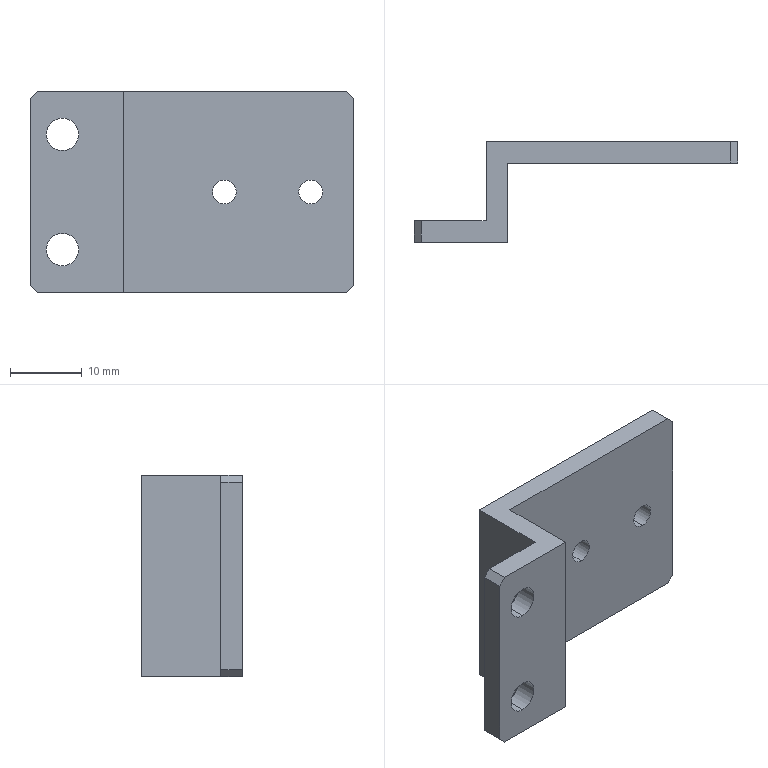Part | NX | features BREP 1 | 1 solid | 22 faces | box 45 x 14 x 28 mm | volume 4551 mm3 | plane 14 | cylinder 8 | commonest cylinder face diameters 3.3 x4 4.5 x4
STEP:
#1=CARTESIAN_POINT('',(103.864,-27.929,12.35));
#2=VERTEX_POINT('',#1);
#3=CARTESIAN_POINT('',(103.864,-27.929,15.65));
#4=VERTEX_POINT('',#3);
#5=CARTESIAN_POINT('',(103.864,-27.929,14.));
#6=DIRECTION('',(0.,1.,0.));
#7=DIRECTION('',(0.,0.,1.));
#8=AXIS2_PLACEMENT_3D('',#5,#6,#7);
#9=CIRCLE('',#8,1.65);
#10=EDGE_CURVE('',#2,#4,#9,.T.);
#11=ORIENTED_EDGE('',*,*,#10,.F.);
#12=CARTESIAN_POINT('',(103.864,-24.929,12.35));
#13=VERTEX_POINT('',#12);
#14=CARTESIAN_POINT('',(103.864,-24.929,12.35));
#15=DIRECTION('',(0.,1.,0.));
#16=VECTOR('',#15,1000.);
#17=LINE('',#14,#16);
#18=EDGE_CURVE('',#13,#2,#17,.F.);
#19=ORIENTED_EDGE('',*,*,#18,.F.);
#20=CARTESIAN_POINT('',(103.864,-24.929,15.65));
#21=VERTEX_POINT('',#20);
#22=CARTESIAN_POINT('',(103.864,-24.929,14.));
#23=DIRECTION('',(0.,1.,0.));
#24=DIRECTION('',(0.,0.,1.));
#25=AXIS2_PLACEMENT_3D('',#22,#23,#24);
#26=CIRCLE('',#25,1.65);
#27=EDGE_CURVE('',#13,#21,#26,.T.);
#28=ORIENTED_EDGE('',*,*,#27,.T.);
#29=CARTESIAN_POINT('',(103.864,-24.929,15.65));
#30=DIRECTION('',(0.,1.,0.));
#31=VECTOR('',#30,1000.);
#32=LINE('',#29,#31);
#33=EDGE_CURVE('',#21,#4,#32,.F.);
#34=ORIENTED_EDGE('',*,*,#33,.T.);
#35=EDGE_LOOP('',(#11,#19,#28,#34));
#36=FACE_BOUND('',#35,.T.);
#37=CARTESIAN_POINT('',(103.864,-24.929,14.));
#38=DIRECTION('',(0.,1.,0.));
#39=DIRECTION('',(0.,0.,1.));
#40=AXIS2_PLACEMENT_3D('',#37,#38,#39);
#41=CYLINDRICAL_SURFACE('',#40,1.65);
#42=ADVANCED_FACE('',(#36),#41,.F.);
#43=CARTESIAN_POINT('',(115.864,-27.929,12.35));
#44=VERTEX_POINT('',#43);
#45=CARTESIAN_POINT('',(115.864,-27.929,15.65));
#46=VERTEX_POINT('',#45);
#47=CARTESIAN_POINT('',(115.864,-27.929,14.));
#48=DIRECTION('',(0.,1.,0.));
#49=DIRECTION('',(0.,0.,1.));
#50=AXIS2_PLACEMENT_3D('',#47,#48,#49);
#51=CIRCLE('',#50,1.65);
#52=EDGE_CURVE('',#44,#46,#51,.T.);
#53=ORIENTED_EDGE('',*,*,#52,.F.);
#54=CARTESIAN_POINT('',(115.864,-24.929,12.35));
#55=VERTEX_POINT('',#54);
#56=CARTESIAN_POINT('',(115.864,-24.929,12.35));
#57=DIRECTION('',(0.,1.,0.));
#58=VECTOR('',#57,1000.);
#59=LINE('',#56,#58);
#60=EDGE_CURVE('',#55,#44,#59,.F.);
#61=ORIENTED_EDGE('',*,*,#60,.F.);
#62=CARTESIAN_POINT('',(115.864,-24.929,15.65));
#63=VERTEX_POINT('',#62);
#64=CARTESIAN_POINT('',(115.864,-24.929,14.));
#65=DIRECTION('',(0.,1.,0.));
#66=DIRECTION('',(0.,0.,1.));
#67=AXIS2_PLACEMENT_3D('',#64,#65,#66);
#68=CIRCLE('',#67,1.65);
#69=EDGE_CURVE('',#55,#63,#68,.T.);
#70=ORIENTED_EDGE('',*,*,#69,.T.);
#71=CARTESIAN_POINT('',(115.864,-24.929,15.65));
#72=DIRECTION('',(0.,1.,0.));
#73=VECTOR('',#72,1000.);
#74=LINE('',#71,#73);
#75=EDGE_CURVE('',#63,#46,#74,.F.);
#76=ORIENTED_EDGE('',*,*,#75,.T.);
#77=EDGE_LOOP('',(#53,#61,#70,#76));
#78=FACE_BOUND('',#77,.T.);
#79=CARTESIAN_POINT('',(115.864,-24.929,14.));
#80=DIRECTION('',(0.,1.,0.));
#81=DIRECTION('',(0.,0.,1.));
#82=AXIS2_PLACEMENT_3D('',#79,#80,#81);
#83=CYLINDRICAL_SURFACE('',#82,1.65);
#84=ADVANCED_FACE('',(#78),#83,.F.);
#85=CARTESIAN_POINT('',(81.364,-38.929,19.75));
#86=VERTEX_POINT('',#85);
#87=CARTESIAN_POINT('',(81.364,-38.929,24.25));
#88=VERTEX_POINT('',#87);
#89=CARTESIAN_POINT('',(81.364,-38.929,22.));
#90=DIRECTION('',(0.,1.,0.));
#91=DIRECTION('',(0.,0.,1.));
#92=AXIS2_PLACEMENT_3D('',#89,#90,#91);
#93=CIRCLE('',#92,2.25);
#94=EDGE_CURVE('',#86,#88,#93,.T.);
#95=ORIENTED_EDGE('',*,*,#94,.F.);
#96=CARTESIAN_POINT('',(81.364,-35.929,19.75));
#97=VERTEX_POINT('',#96);
#98=CARTESIAN_POINT('',(81.364,-38.929,19.75));
#99=DIRECTION('',(0.,1.,0.));
#100=VECTOR('',#99,1000.);
#101=LINE('',#98,#100);
#102=EDGE_CURVE('',#97,#86,#101,.F.);
#103=ORIENTED_EDGE('',*,*,#102,.F.);
#104=CARTESIAN_POINT('',(81.364,-35.929,24.25));
#105=VERTEX_POINT('',#104);
#106=CARTESIAN_POINT('',(81.364,-35.929,22.));
#107=DIRECTION('',(0.,1.,0.));
#108=DIRECTION('',(0.,0.,1.));
#109=AXIS2_PLACEMENT_3D('',#106,#107,#108);
#110=CIRCLE('',#109,2.25);
#111=EDGE_CURVE('',#97,#105,#110,.T.);
#112=ORIENTED_EDGE('',*,*,#111,.T.);
#113=CARTESIAN_POINT('',(81.364,-38.929,24.25));
#114=DIRECTION('',(0.,1.,0.));
#115=VECTOR('',#114,1000.);
#116=LINE('',#113,#115);
#117=EDGE_CURVE('',#105,#88,#116,.F.);
#118=ORIENTED_EDGE('',*,*,#117,.T.);
#119=EDGE_LOOP('',(#95,#103,#112,#118));
#120=FACE_BOUND('',#119,.T.);
#121=CARTESIAN_POINT('',(81.364,-38.929,22.));
#122=DIRECTION('',(0.,1.,0.));
#123=DIRECTION('',(0.,0.,1.));
#124=AXIS2_PLACEMENT_3D('',#121,#122,#123);
#125=CYLINDRICAL_SURFACE('',#124,2.25);
#126=ADVANCED_FACE('',(#120),#125,.F.);
#127=CARTESIAN_POINT('',(81.364,-38.929,3.75));
#128=VERTEX_POINT('',#127);
#129=CARTESIAN_POINT('',(81.364,-38.929,8.25));
#130=VERTEX_POINT('',#129);
#131=CARTESIAN_POINT('',(81.364,-38.929,6.));
#132=DIRECTION('',(0.,1.,0.));
#133=DIRECTION('',(0.,0.,1.));
#134=AXIS2_PLACEMENT_3D('',#131,#132,#133);
#135=CIRCLE('',#134,2.25);
#136=EDGE_CURVE('',#128,#130,#135,.T.);
#137=ORIENTED_EDGE('',*,*,#136,.F.);
#138=CARTESIAN_POINT('',(81.364,-35.929,3.75));
#139=VERTEX_POINT('',#138);
#140=CARTESIAN_POINT('',(81.364,-38.929,3.75));
#141=DIRECTION('',(0.,1.,0.));
#142=VECTOR('',#141,1000.);
#143=LINE('',#140,#142);
#144=EDGE_CURVE('',#139,#128,#143,.F.);
#145=ORIENTED_EDGE('',*,*,#144,.F.);
#146=CARTESIAN_POINT('',(81.364,-35.929,8.25));
#147=VERTEX_POINT('',#146);
#148=CARTESIAN_POINT('',(81.364,-35.929,6.));
#149=DIRECTION('',(0.,1.,0.));
#150=DIRECTION('',(0.,0.,1.));
#151=AXIS2_PLACEMENT_3D('',#148,#149,#150);
#152=CIRCLE('',#151,2.25);
#153=EDGE_CURVE('',#139,#147,#152,.T.);
#154=ORIENTED_EDGE('',*,*,#153,.T.);
#155=CARTESIAN_POINT('',(81.364,-38.929,8.25));
#156=DIRECTION('',(0.,1.,0.));
#157=VECTOR('',#156,1000.);
#158=LINE('',#155,#157);
#159=EDGE_CURVE('',#147,#130,#158,.F.);
#160=ORIENTED_EDGE('',*,*,#159,.T.);
#161=EDGE_LOOP('',(#137,#145,#154,#160));
#162=FACE_BOUND('',#161,.T.);
#163=CARTESIAN_POINT('',(81.364,-38.929,6.));
#164=DIRECTION('',(0.,1.,0.));
#165=DIRECTION('',(0.,0.,1.));
#166=AXIS2_PLACEMENT_3D('',#163,#164,#165);
#167=CYLINDRICAL_SURFACE('',#166,2.25);
#168=ADVANCED_FACE('',(#162),#167,.F.);
#169=CARTESIAN_POINT('',(86.864,-24.929,0.));
#170=VERTEX_POINT('',#169);
#171=CARTESIAN_POINT('',(86.864,-35.929,0.));
#172=VERTEX_POINT('',#171);
#173=CARTESIAN_POINT('',(86.864,-24.929,0.));
#174=DIRECTION('',(0.,-1.,0.));
#175=VECTOR('',#174,1000.);
#176=LINE('',#173,#175);
#177=EDGE_CURVE('',#170,#172,#176,.T.);
#178=ORIENTED_EDGE('',*,*,#177,.T.);
#179=CARTESIAN_POINT('',(86.864,-35.929,28.));
#180=VERTEX_POINT('',#179);
#181=CARTESIAN_POINT('',(86.864,-35.929,28.));
#182=DIRECTION('',(0.,0.,-1.));
#183=VECTOR('',#182,1000.);
#184=LINE('',#181,#183);
#185=EDGE_CURVE('',#180,#172,#184,.T.);
#186=ORIENTED_EDGE('',*,*,#185,.F.);
#187=CARTESIAN_POINT('',(86.864,-24.929,28.));
#188=VERTEX_POINT('',#187);
#189=CARTESIAN_POINT('',(86.864,-24.929,28.));
#190=DIRECTION('',(0.,-1.,0.));
#191=VECTOR('',#190,1000.);
#192=LINE('',#189,#191);
#193=EDGE_CURVE('',#188,#180,#192,.T.);
#194=ORIENTED_EDGE('',*,*,#193,.F.);
#195=CARTESIAN_POINT('',(86.864,-24.929,28.));
#196=DIRECTION('',(0.,0.,-1.));
#197=VECTOR('',#196,1000.);
#198=LINE('',#195,#197);
#199=EDGE_CURVE('',#188,#170,#198,.T.);
#200=ORIENTED_EDGE('',*,*,#199,.T.);
#201=EDGE_LOOP('',(#178,#186,#194,#200));
#202=FACE_BOUND('',#201,.T.);
#203=CARTESIAN_POINT('',(86.864,-24.929,28.));
#204=DIRECTION('',(1.,0.,0.));
#205=DIRECTION('',(0.,1.,0.));
#206=AXIS2_PLACEMENT_3D('',#203,#204,#205);
#207=PLANE('',#206);
#208=ADVANCED_FACE('',(#202),#207,.F.);
#209=CARTESIAN_POINT('',(77.864,-35.929,0.));
#210=VERTEX_POINT('',#209);
#211=CARTESIAN_POINT('',(86.864,-35.929,0.));
#212=DIRECTION('',(-1.,0.,0.));
#213=VECTOR('',#212,1000.);
#214=LINE('',#211,#213);
#215=EDGE_CURVE('',#172,#210,#214,.T.);
#216=ORIENTED_EDGE('',*,*,#215,.T.);
#217=CARTESIAN_POINT('',(76.864,-35.929,1.));
#218=VERTEX_POINT('',#217);
#219=CARTESIAN_POINT('',(76.864,-35.929,1.));
#220=DIRECTION('',(-0.7071,0.,0.7071));
#221=VECTOR('',#220,1000.);
#222=LINE('',#219,#221);
#223=EDGE_CURVE('',#210,#218,#222,.T.);
#224=ORIENTED_EDGE('',*,*,#223,.T.);
#225=CARTESIAN_POINT('',(76.864,-35.929,27.));
#226=VERTEX_POINT('',#225);
#227=CARTESIAN_POINT('',(76.864,-35.929,28.));
#228=DIRECTION('',(0.,0.,-1.));
#229=VECTOR('',#228,1000.);
#230=LINE('',#227,#229);
#231=EDGE_CURVE('',#226,#218,#230,.T.);
#232=ORIENTED_EDGE('',*,*,#231,.F.);
#233=CARTESIAN_POINT('',(77.864,-35.929,28.));
#234=VERTEX_POINT('',#233);
#235=CARTESIAN_POINT('',(77.864,-35.929,28.));
#236=DIRECTION('',(0.7071,0.,0.7071));
#237=VECTOR('',#236,1000.);
#238=LINE('',#235,#237);
#239=EDGE_CURVE('',#226,#234,#238,.T.);
#240=ORIENTED_EDGE('',*,*,#239,.T.);
#241=CARTESIAN_POINT('',(86.864,-35.929,28.));
#242=DIRECTION('',(-1.,0.,0.));
#243=VECTOR('',#242,1000.);
#244=LINE('',#241,#243);
#245=EDGE_CURVE('',#180,#234,#244,.T.);
#246=ORIENTED_EDGE('',*,*,#245,.F.);
#247=ORIENTED_EDGE('',*,*,#185,.T.);
#248=EDGE_LOOP('',(#216,#224,#232,#240,#246,#247));
#249=FACE_BOUND('',#248,.T.);
#250=CARTESIAN_POINT('',(81.364,-35.929,22.));
#251=DIRECTION('',(0.,1.,0.));
#252=DIRECTION('',(0.,0.,1.));
#253=AXIS2_PLACEMENT_3D('',#250,#251,#252);
#254=CIRCLE('',#253,2.25);
#255=EDGE_CURVE('',#105,#97,#254,.T.);
#256=ORIENTED_EDGE('',*,*,#255,.F.);
#257=ORIENTED_EDGE('',*,*,#111,.F.);
#258=EDGE_LOOP('',(#256,#257));
#259=FACE_BOUND('',#258,.T.);
#260=CARTESIAN_POINT('',(81.364,-35.929,6.));
#261=DIRECTION('',(0.,1.,0.));
#262=DIRECTION('',(0.,0.,1.));
#263=AXIS2_PLACEMENT_3D('',#260,#261,#262);
#264=CIRCLE('',#263,2.25);
#265=EDGE_CURVE('',#147,#139,#264,.T.);
#266=ORIENTED_EDGE('',*,*,#265,.F.);
#267=ORIENTED_EDGE('',*,*,#153,.F.);
#268=EDGE_LOOP('',(#266,#267));
#269=FACE_BOUND('',#268,.T.);
#270=CARTESIAN_POINT('',(86.864,-35.929,28.));
#271=DIRECTION('',(0.,-1.,0.));
#272=DIRECTION('',(0.,0.,-1.));
#273=AXIS2_PLACEMENT_3D('',#270,#271,#272);
#274=PLANE('',#273);
#275=ADVANCED_FACE('',(#249,#259,#269),#274,.F.);
#276=ORIENTED_EDGE('',*,*,#231,.T.);
#277=CARTESIAN_POINT('',(76.864,-38.929,1.));
#278=VERTEX_POINT('',#277);
#279=CARTESIAN_POINT('',(76.864,-38.929,1.));
#280=DIRECTION('',(0.,-1.,0.));
#281=VECTOR('',#280,1000.);
#282=LINE('',#279,#281);
#283=EDGE_CURVE('',#218,#278,#282,.T.);
#284=ORIENTED_EDGE('',*,*,#283,.T.);
#285=CARTESIAN_POINT('',(76.864,-38.929,27.));
#286=VERTEX_POINT('',#285);
#287=CARTESIAN_POINT('',(76.864,-38.929,28.));
#288=DIRECTION('',(0.,0.,-1.));
#289=VECTOR('',#288,1000.);
#290=LINE('',#287,#289);
#291=EDGE_CURVE('',#286,#278,#290,.T.);
#292=ORIENTED_EDGE('',*,*,#291,.F.);
#293=CARTESIAN_POINT('',(76.864,-35.929,27.));
#294=DIRECTION('',(0.,1.,0.));
#295=VECTOR('',#294,1000.);
#296=LINE('',#293,#295);
#297=EDGE_CURVE('',#286,#226,#296,.T.);
#298=ORIENTED_EDGE('',*,*,#297,.T.);
#299=EDGE_LOOP('',(#276,#284,#292,#298));
#300=FACE_BOUND('',#299,.T.);
#301=CARTESIAN_POINT('',(76.864,-35.929,28.));
#302=DIRECTION('',(1.,0.,0.));
#303=DIRECTION('',(0.,1.,0.));
#304=AXIS2_PLACEMENT_3D('',#301,#302,#303);
#305=PLANE('',#304);
#306=ADVANCED_FACE('',(#300),#305,.F.);
#307=ORIENTED_EDGE('',*,*,#291,.T.);
#308=CARTESIAN_POINT('',(77.864,-38.929,0.));
#309=VERTEX_POINT('',#308);
#310=CARTESIAN_POINT('',(76.864,-38.929,1.));
#311=DIRECTION('',(0.7071,0.,-0.7071));
#312=VECTOR('',#311,1000.);
#313=LINE('',#310,#312);
#314=EDGE_CURVE('',#278,#309,#313,.T.);
#315=ORIENTED_EDGE('',*,*,#314,.T.);
#316=CARTESIAN_POINT('',(89.864,-38.929,0.));
#317=VERTEX_POINT('',#316);
#318=CARTESIAN_POINT('',(89.864,-38.929,0.));
#319=DIRECTION('',(1.,0.,0.));
#320=VECTOR('',#319,1000.);
#321=LINE('',#318,#320);
#322=EDGE_CURVE('',#309,#317,#321,.T.);
#323=ORIENTED_EDGE('',*,*,#322,.T.);
#324=CARTESIAN_POINT('',(89.864,-38.929,28.));
#325=VERTEX_POINT('',#324);
#326=CARTESIAN_POINT('',(89.864,-38.929,28.));
#327=DIRECTION('',(0.,0.,-1.));
#328=VECTOR('',#327,1000.);
#329=LINE('',#326,#328);
#330=EDGE_CURVE('',#325,#317,#329,.T.);
#331=ORIENTED_EDGE('',*,*,#330,.F.);
#332=CARTESIAN_POINT('',(77.864,-38.929,28.));
#333=VERTEX_POINT('',#332);
#334=CARTESIAN_POINT('',(89.864,-38.929,28.));
#335=DIRECTION('',(1.,0.,0.));
#336=VECTOR('',#335,1000.);
#337=LINE('',#334,#336);
#338=EDGE_CURVE('',#333,#325,#337,.T.);
#339=ORIENTED_EDGE('',*,*,#338,.F.);
#340=CARTESIAN_POINT('',(77.864,-38.929,28.));
#341=DIRECTION('',(-0.7071,0.,-0.7071));
#342=VECTOR('',#341,1000.);
#343=LINE('',#340,#342);
#344=EDGE_CURVE('',#333,#286,#343,.T.);
#345=ORIENTED_EDGE('',*,*,#344,.T.);
#346=EDGE_LOOP('',(#307,#315,#323,#331,#339,#345));
#347=FACE_BOUND('',#346,.T.);
#348=CARTESIAN_POINT('',(81.364,-38.929,22.));
#349=DIRECTION('',(0.,1.,0.));
#350=DIRECTION('',(0.,0.,1.));
#351=AXIS2_PLACEMENT_3D('',#348,#349,#350);
#352=CIRCLE('',#351,2.25);
#353=EDGE_CURVE('',#88,#86,#352,.T.);
#354=ORIENTED_EDGE('',*,*,#353,.T.);
#355=ORIENTED_EDGE('',*,*,#94,.T.);
#356=EDGE_LOOP('',(#354,#355));
#357=FACE_BOUND('',#356,.T.);
#358=CARTESIAN_POINT('',(81.364,-38.929,6.));
#359=DIRECTION('',(0.,1.,0.));
#360=DIRECTION('',(0.,0.,1.));
#361=AXIS2_PLACEMENT_3D('',#358,#359,#360);
#362=CIRCLE('',#361,2.25);
#363=EDGE_CURVE('',#130,#128,#362,.T.);
#364=ORIENTED_EDGE('',*,*,#363,.T.);
#365=ORIENTED_EDGE('',*,*,#136,.T.);
#366=EDGE_LOOP('',(#364,#365));
#367=FACE_BOUND('',#366,.T.);
#368=CARTESIAN_POINT('',(89.864,-38.929,28.));
#369=DIRECTION('',(0.,1.,0.));
#370=DIRECTION('',(1.,0.,0.));
#371=AXIS2_PLACEMENT_3D('',#368,#369,#370);
#372=PLANE('',#371);
#373=ADVANCED_FACE('',(#347,#357,#367),#372,.F.);
#374=CARTESIAN_POINT('',(89.864,-27.929,0.));
#375=VERTEX_POINT('',#374);
#376=CARTESIAN_POINT('',(89.864,-27.929,0.));
#377=DIRECTION('',(0.,1.,0.));
#378=VECTOR('',#377,1000.);
#379=LINE('',#376,#378);
#380=EDGE_CURVE('',#317,#375,#379,.T.);
#381=ORIENTED_EDGE('',*,*,#380,.T.);
#382=CARTESIAN_POINT('',(89.864,-27.929,28.));
#383=VERTEX_POINT('',#382);
#384=CARTESIAN_POINT('',(89.864,-27.929,28.));
#385=DIRECTION('',(0.,0.,-1.));
#386=VECTOR('',#385,1000.);
#387=LINE('',#384,#386);
#388=EDGE_CURVE('',#383,#375,#387,.T.);
#389=ORIENTED_EDGE('',*,*,#388,.F.);
#390=CARTESIAN_POINT('',(89.864,-27.929,28.));
#391=DIRECTION('',(0.,1.,0.));
#392=VECTOR('',#391,1000.);
#393=LINE('',#390,#392);
#394=EDGE_CURVE('',#325,#383,#393,.T.);
#395=ORIENTED_EDGE('',*,*,#394,.F.);
#396=ORIENTED_EDGE('',*,*,#330,.T.);
#397=EDGE_LOOP('',(#381,#389,#395,#396));
#398=FACE_BOUND('',#397,.T.);
#399=CARTESIAN_POINT('',(89.864,-27.929,28.));
#400=DIRECTION('',(-1.,0.,0.));
#401=DIRECTION('',(0.,0.,1.));
#402=AXIS2_PLACEMENT_3D('',#399,#400,#401);
#403=PLANE('',#402);
#404=ADVANCED_FACE('',(#398),#403,.F.);
#405=CARTESIAN_POINT('',(120.864,-27.929,0.));
#406=VERTEX_POINT('',#405);
#407=CARTESIAN_POINT('',(89.864,-27.929,0.));
#408=DIRECTION('',(1.,0.,0.));
#409=VECTOR('',#408,1000.);
#410=LINE('',#407,#409);
#411=EDGE_CURVE('',#375,#406,#410,.T.);
#412=ORIENTED_EDGE('',*,*,#411,.T.);
#413=CARTESIAN_POINT('',(121.864,-27.929,1.));
#414=VERTEX_POINT('',#413);
#415=CARTESIAN_POINT('',(121.864,-27.929,1.));
#416=DIRECTION('',(0.7071,0.,0.7071));
#417=VECTOR('',#416,1000.);
#418=LINE('',#415,#417);
#419=EDGE_CURVE('',#406,#414,#418,.T.);
#420=ORIENTED_EDGE('',*,*,#419,.T.);
#421=CARTESIAN_POINT('',(121.864,-27.929,27.));
#422=VERTEX_POINT('',#421);
#423=CARTESIAN_POINT('',(121.864,-27.929,28.));
#424=DIRECTION('',(0.,0.,-1.));
#425=VECTOR('',#424,1000.);
#426=LINE('',#423,#425);
#427=EDGE_CURVE('',#422,#414,#426,.T.);
#428=ORIENTED_EDGE('',*,*,#427,.F.);
#429=CARTESIAN_POINT('',(120.864,-27.929,28.));
#430=VERTEX_POINT('',#429);
#431=CARTESIAN_POINT('',(120.864,-27.929,28.));
#432=DIRECTION('',(-0.7071,0.,0.7071));
#433=VECTOR('',#432,1000.);
#434=LINE('',#431,#433);
#435=EDGE_CURVE('',#422,#430,#434,.T.);
#436=ORIENTED_EDGE('',*,*,#435,.T.);
#437=CARTESIAN_POINT('',(89.864,-27.929,28.));
#438=DIRECTION('',(1.,0.,0.));
#439=VECTOR('',#438,1000.);
#440=LINE('',#437,#439);
#441=EDGE_CURVE('',#383,#430,#440,.T.);
#442=ORIENTED_EDGE('',*,*,#441,.F.);
#443=ORIENTED_EDGE('',*,*,#388,.T.);
#444=EDGE_LOOP('',(#412,#420,#428,#436,#442,#443));
#445=FACE_BOUND('',#444,.T.);
#446=CARTESIAN_POINT('',(103.864,-27.929,14.));
#447=DIRECTION('',(0.,1.,0.));
#448=DIRECTION('',(0.,0.,1.));
#449=AXIS2_PLACEMENT_3D('',#446,#447,#448);
#450=CIRCLE('',#449,1.65);
#451=EDGE_CURVE('',#4,#2,#450,.T.);
#452=ORIENTED_EDGE('',*,*,#451,.T.);
#453=ORIENTED_EDGE('',*,*,#10,.T.);
#454=EDGE_LOOP('',(#452,#453));
#455=FACE_BOUND('',#454,.T.);
#456=CARTESIAN_POINT('',(115.864,-27.929,14.));
#457=DIRECTION('',(0.,1.,0.));
#458=DIRECTION('',(0.,0.,1.));
#459=AXIS2_PLACEMENT_3D('',#456,#457,#458);
#460=CIRCLE('',#459,1.65);
#461=EDGE_CURVE('',#46,#44,#460,.T.);
#462=ORIENTED_EDGE('',*,*,#461,.T.);
#463=ORIENTED_EDGE('',*,*,#52,.T.);
#464=EDGE_LOOP('',(#462,#463));
#465=FACE_BOUND('',#464,.T.);
#466=CARTESIAN_POINT('',(89.864,-27.929,28.));
#467=DIRECTION('',(0.,1.,0.));
#468=DIRECTION('',(1.,0.,0.));
#469=AXIS2_PLACEMENT_3D('',#466,#467,#468);
#470=PLANE('',#469);
#471=ADVANCED_FACE('',(#445,#455,#465),#470,.F.);
#472=ORIENTED_EDGE('',*,*,#427,.T.);
#473=CARTESIAN_POINT('',(121.864,-24.929,1.));
#474=VERTEX_POINT('',#473);
#475=CARTESIAN_POINT('',(121.864,-24.929,1.));
#476=DIRECTION('',(0.,1.,0.));
#477=VECTOR('',#476,1000.);
#478=LINE('',#475,#477);
#479=EDGE_CURVE('',#414,#474,#478,.T.);
#480=ORIENTED_EDGE('',*,*,#479,.T.);
#481=CARTESIAN_POINT('',(121.864,-24.929,27.));
#482=VERTEX_POINT('',#481);
#483=CARTESIAN_POINT('',(121.864,-24.929,28.));
#484=DIRECTION('',(0.,0.,-1.));
#485=VECTOR('',#484,1000.);
#486=LINE('',#483,#485);
#487=EDGE_CURVE('',#482,#474,#486,.T.);
#488=ORIENTED_EDGE('',*,*,#487,.F.);
#489=CARTESIAN_POINT('',(121.864,-24.929,27.));
#490=DIRECTION('',(0.,-1.,0.));
#491=VECTOR('',#490,1000.);
#492=LINE('',#489,#491);
#493=EDGE_CURVE('',#482,#422,#492,.T.);
#494=ORIENTED_EDGE('',*,*,#493,.T.);
#495=EDGE_LOOP('',(#472,#480,#488,#494));
#496=FACE_BOUND('',#495,.T.);
#497=CARTESIAN_POINT('',(121.864,-24.929,28.));
#498=DIRECTION('',(-1.,0.,0.));
#499=DIRECTION('',(0.,0.,1.));
#500=AXIS2_PLACEMENT_3D('',#497,#498,#499);
#501=PLANE('',#500);
#502=ADVANCED_FACE('',(#496),#501,.F.);
#503=ORIENTED_EDGE('',*,*,#487,.T.);
#504=CARTESIAN_POINT('',(120.864,-24.929,0.));
#505=VERTEX_POINT('',#504);
#506=CARTESIAN_POINT('',(121.864,-24.929,1.));
#507=DIRECTION('',(-0.7071,0.,-0.7071));
#508=VECTOR('',#507,1000.);
#509=LINE('',#506,#508);
#510=EDGE_CURVE('',#474,#505,#509,.T.);
#511=ORIENTED_EDGE('',*,*,#510,.T.);
#512=CARTESIAN_POINT('',(86.864,-24.929,0.));
#513=DIRECTION('',(-1.,0.,0.));
#514=VECTOR('',#513,1000.);
#515=LINE('',#512,#514);
#516=EDGE_CURVE('',#505,#170,#515,.T.);
#517=ORIENTED_EDGE('',*,*,#516,.T.);
#518=ORIENTED_EDGE('',*,*,#199,.F.);
#519=CARTESIAN_POINT('',(120.864,-24.929,28.));
#520=VERTEX_POINT('',#519);
#521=CARTESIAN_POINT('',(86.864,-24.929,28.));
#522=DIRECTION('',(-1.,0.,0.));
#523=VECTOR('',#522,1000.);
#524=LINE('',#521,#523);
#525=EDGE_CURVE('',#520,#188,#524,.T.);
#526=ORIENTED_EDGE('',*,*,#525,.F.);
#527=CARTESIAN_POINT('',(120.864,-24.929,28.));
#528=DIRECTION('',(0.7071,0.,-0.7071));
#529=VECTOR('',#528,1000.);
#530=LINE('',#527,#529);
#531=EDGE_CURVE('',#520,#482,#530,.T.);
#532=ORIENTED_EDGE('',*,*,#531,.T.);
#533=EDGE_LOOP('',(#503,#511,#517,#518,#526,#532));
#534=FACE_BOUND('',#533,.T.);
#535=CARTESIAN_POINT('',(103.864,-24.929,14.));
#536=DIRECTION('',(0.,1.,0.));
#537=DIRECTION('',(0.,0.,1.));
#538=AXIS2_PLACEMENT_3D('',#535,#536,#537);
#539=CIRCLE('',#538,1.65);
#540=EDGE_CURVE('',#21,#13,#539,.T.);
#541=ORIENTED_EDGE('',*,*,#540,.F.);
#542=ORIENTED_EDGE('',*,*,#27,.F.);
#543=EDGE_LOOP('',(#541,#542));
#544=FACE_BOUND('',#543,.T.);
#545=CARTESIAN_POINT('',(115.864,-24.929,14.));
#546=DIRECTION('',(0.,1.,0.));
#547=DIRECTION('',(0.,0.,1.));
#548=AXIS2_PLACEMENT_3D('',#545,#546,#547);
#549=CIRCLE('',#548,1.65);
#550=EDGE_CURVE('',#63,#55,#549,.T.);
#551=ORIENTED_EDGE('',*,*,#550,.F.);
#552=ORIENTED_EDGE('',*,*,#69,.F.);
#553=EDGE_LOOP('',(#551,#552));
#554=FACE_BOUND('',#553,.T.);
#555=CARTESIAN_POINT('',(86.864,-24.929,28.));
#556=DIRECTION('',(0.,-1.,0.));
#557=DIRECTION('',(0.,0.,-1.));
#558=AXIS2_PLACEMENT_3D('',#555,#556,#557);
#559=PLANE('',#558);
#560=ADVANCED_FACE('',(#534,#544,#554),#559,.F.);
#561=ORIENTED_EDGE('',*,*,#441,.T.);
#562=CARTESIAN_POINT('',(120.864,-35.929,28.));
#563=DIRECTION('',(0.,1.,0.));
#564=VECTOR('',#563,1000.);
#565=LINE('',#562,#564);
#566=EDGE_CURVE('',#430,#520,#565,.T.);
#567=ORIENTED_EDGE('',*,*,#566,.T.);
#568=ORIENTED_EDGE('',*,*,#525,.T.);
#569=ORIENTED_EDGE('',*,*,#193,.T.);
#570=ORIENTED_EDGE('',*,*,#245,.T.);
#571=CARTESIAN_POINT('',(77.864,-35.929,28.));
#572=DIRECTION('',(0.,-1.,0.));
#573=VECTOR('',#572,1000.);
#574=LINE('',#571,#573);
#575=EDGE_CURVE('',#234,#333,#574,.T.);
#576=ORIENTED_EDGE('',*,*,#575,.T.);
#577=ORIENTED_EDGE('',*,*,#338,.T.);
#578=ORIENTED_EDGE('',*,*,#394,.T.);
#579=EDGE_LOOP('',(#561,#567,#568,#569,#570,#576,#577,#578));
#580=FACE_BOUND('',#579,.T.);
#581=CARTESIAN_POINT('',(86.864,-35.929,28.));
#582=DIRECTION('',(0.,0.,-1.));
#583=DIRECTION('',(0.,-1.,0.));
#584=AXIS2_PLACEMENT_3D('',#581,#582,#583);
#585=PLANE('',#584);
#586=ADVANCED_FACE('',(#580),#585,.F.);
#587=ORIENTED_EDGE('',*,*,#516,.F.);
#588=CARTESIAN_POINT('',(120.864,-27.929,0.));
#589=DIRECTION('',(0.,-1.,0.));
#590=VECTOR('',#589,1000.);
#591=LINE('',#588,#590);
#592=EDGE_CURVE('',#505,#406,#591,.T.);
#593=ORIENTED_EDGE('',*,*,#592,.T.);
#594=ORIENTED_EDGE('',*,*,#411,.F.);
#595=ORIENTED_EDGE('',*,*,#380,.F.);
#596=ORIENTED_EDGE('',*,*,#322,.F.);
#597=CARTESIAN_POINT('',(77.864,-35.929,0.));
#598=DIRECTION('',(0.,1.,0.));
#599=VECTOR('',#598,1000.);
#600=LINE('',#597,#599);
#601=EDGE_CURVE('',#309,#210,#600,.T.);
#602=ORIENTED_EDGE('',*,*,#601,.T.);
#603=ORIENTED_EDGE('',*,*,#215,.F.);
#604=ORIENTED_EDGE('',*,*,#177,.F.);
#605=EDGE_LOOP('',(#587,#593,#594,#595,#596,#602,#603,#604));
#606=FACE_BOUND('',#605,.T.);
#607=CARTESIAN_POINT('',(86.864,-35.929,0.));
#608=DIRECTION('',(0.,0.,-1.));
#609=DIRECTION('',(0.,-1.,0.));
#610=AXIS2_PLACEMENT_3D('',#607,#608,#609);
#611=PLANE('',#610);
#612=ADVANCED_FACE('',(#606),#611,.T.);
#613=ORIENTED_EDGE('',*,*,#144,.T.);
#614=ORIENTED_EDGE('',*,*,#363,.F.);
#615=ORIENTED_EDGE('',*,*,#159,.F.);
#616=ORIENTED_EDGE('',*,*,#265,.T.);
#617=EDGE_LOOP('',(#613,#614,#615,#616));
#618=FACE_BOUND('',#617,.T.);
#619=CARTESIAN_POINT('',(81.364,-38.929,6.));
#620=DIRECTION('',(0.,1.,0.));
#621=DIRECTION('',(0.,0.,1.));
#622=AXIS2_PLACEMENT_3D('',#619,#620,#621);
#623=CYLINDRICAL_SURFACE('',#622,2.25);
#624=ADVANCED_FACE('',(#618),#623,.F.);
#625=ORIENTED_EDGE('',*,*,#102,.T.);
#626=ORIENTED_EDGE('',*,*,#353,.F.);
#627=ORIENTED_EDGE('',*,*,#117,.F.);
#628=ORIENTED_EDGE('',*,*,#255,.T.);
#629=EDGE_LOOP('',(#625,#626,#627,#628));
#630=FACE_BOUND('',#629,.T.);
#631=CARTESIAN_POINT('',(81.364,-38.929,22.));
#632=DIRECTION('',(0.,1.,0.));
#633=DIRECTION('',(0.,0.,1.));
#634=AXIS2_PLACEMENT_3D('',#631,#632,#633);
#635=CYLINDRICAL_SURFACE('',#634,2.25);
#636=ADVANCED_FACE('',(#630),#635,.F.);
#637=ORIENTED_EDGE('',*,*,#60,.T.);
#638=ORIENTED_EDGE('',*,*,#461,.F.);
#639=ORIENTED_EDGE('',*,*,#75,.F.);
#640=ORIENTED_EDGE('',*,*,#550,.T.);
#641=EDGE_LOOP('',(#637,#638,#639,#640));
#642=FACE_BOUND('',#641,.T.);
#643=CARTESIAN_POINT('',(115.864,-24.929,14.));
#644=DIRECTION('',(0.,1.,0.));
#645=DIRECTION('',(0.,0.,1.));
#646=AXIS2_PLACEMENT_3D('',#643,#644,#645);
#647=CYLINDRICAL_SURFACE('',#646,1.65);
#648=ADVANCED_FACE('',(#642),#647,.F.);
#649=ORIENTED_EDGE('',*,*,#18,.T.);
#650=ORIENTED_EDGE('',*,*,#451,.F.);
#651=ORIENTED_EDGE('',*,*,#33,.F.);
#652=ORIENTED_EDGE('',*,*,#540,.T.);
#653=EDGE_LOOP('',(#649,#650,#651,#652));
#654=FACE_BOUND('',#653,.T.);
#655=CARTESIAN_POINT('',(103.864,-24.929,14.));
#656=DIRECTION('',(0.,1.,0.));
#657=DIRECTION('',(0.,0.,1.));
#658=AXIS2_PLACEMENT_3D('',#655,#656,#657);
#659=CYLINDRICAL_SURFACE('',#658,1.65);
#660=ADVANCED_FACE('',(#654),#659,.F.);
#661=ORIENTED_EDGE('',*,*,#419,.F.);
#662=ORIENTED_EDGE('',*,*,#592,.F.);
#663=ORIENTED_EDGE('',*,*,#510,.F.);
#664=ORIENTED_EDGE('',*,*,#479,.F.);
#665=EDGE_LOOP('',(#661,#662,#663,#664));
#666=FACE_BOUND('',#665,.T.);
#667=CARTESIAN_POINT('',(121.864,-24.929,1.));
#668=DIRECTION('',(0.7071,0.,-0.7071));
#669=DIRECTION('',(0.,-1.,0.));
#670=AXIS2_PLACEMENT_3D('',#667,#668,#669);
#671=PLANE('',#670);
#672=ADVANCED_FACE('',(#666),#671,.T.);
#673=ORIENTED_EDGE('',*,*,#435,.F.);
#674=ORIENTED_EDGE('',*,*,#493,.F.);
#675=ORIENTED_EDGE('',*,*,#531,.F.);
#676=ORIENTED_EDGE('',*,*,#566,.F.);
#677=EDGE_LOOP('',(#673,#674,#675,#676));
#678=FACE_BOUND('',#677,.T.);
#679=CARTESIAN_POINT('',(120.864,-35.929,28.));
#680=DIRECTION('',(-0.7071,0.,-0.7071));
#681=DIRECTION('',(-0.7071,0.,0.7071));
#682=AXIS2_PLACEMENT_3D('',#679,#680,#681);
#683=PLANE('',#682);
#684=ADVANCED_FACE('',(#678),#683,.F.);
#685=ORIENTED_EDGE('',*,*,#223,.F.);
#686=ORIENTED_EDGE('',*,*,#601,.F.);
#687=ORIENTED_EDGE('',*,*,#314,.F.);
#688=ORIENTED_EDGE('',*,*,#283,.F.);
#689=EDGE_LOOP('',(#685,#686,#687,#688));
#690=FACE_BOUND('',#689,.T.);
#691=CARTESIAN_POINT('',(76.864,-35.929,1.));
#692=DIRECTION('',(-0.7071,0.,-0.7071));
#693=DIRECTION('',(-0.7071,0.,0.7071));
#694=AXIS2_PLACEMENT_3D('',#691,#692,#693);
#695=PLANE('',#694);
#696=ADVANCED_FACE('',(#690),#695,.T.);
#697=ORIENTED_EDGE('',*,*,#239,.F.);
#698=ORIENTED_EDGE('',*,*,#297,.F.);
#699=ORIENTED_EDGE('',*,*,#344,.F.);
#700=ORIENTED_EDGE('',*,*,#575,.F.);
#701=EDGE_LOOP('',(#697,#698,#699,#700));
#702=FACE_BOUND('',#701,.T.);
#703=CARTESIAN_POINT('',(77.864,-35.929,28.));
#704=DIRECTION('',(0.7071,0.,-0.7071));
#705=DIRECTION('',(0.,-1.,0.));
#706=AXIS2_PLACEMENT_3D('',#703,#704,#705);
#707=PLANE('',#706);
#708=ADVANCED_FACE('',(#702),#707,.F.);
#709=CLOSED_SHELL('',(#42,#84,#126,#168,#208,#275,#306,#373,#404,#471,#502,#560,#586,#612,#624,#636,#648,#660,#672,#684,#696,#708));
#710=MANIFOLD_SOLID_BREP('',#709);
#711=(LENGTH_UNIT()NAMED_UNIT(*)SI_UNIT(.MILLI.,.METRE.));
#712=UNCERTAINTY_MEASURE_WITH_UNIT(LENGTH_MEASURE(0.00001),#711,'','');
#713=(NAMED_UNIT(*)PLANE_ANGLE_UNIT()SI_UNIT($,.RADIAN.));
#714=(NAMED_UNIT(*)SI_UNIT($,.STERADIAN.)SOLID_ANGLE_UNIT());
#715=(GEOMETRIC_REPRESENTATION_CONTEXT(3)GLOBAL_UNCERTAINTY_ASSIGNED_CONTEXT((#712))GLOBAL_UNIT_ASSIGNED_CONTEXT((#711,#713,#714))REPRESENTATION_CONTEXT('',''));
#716=ADVANCED_BREP_SHAPE_REPRESENTATION('',(#710),#715);